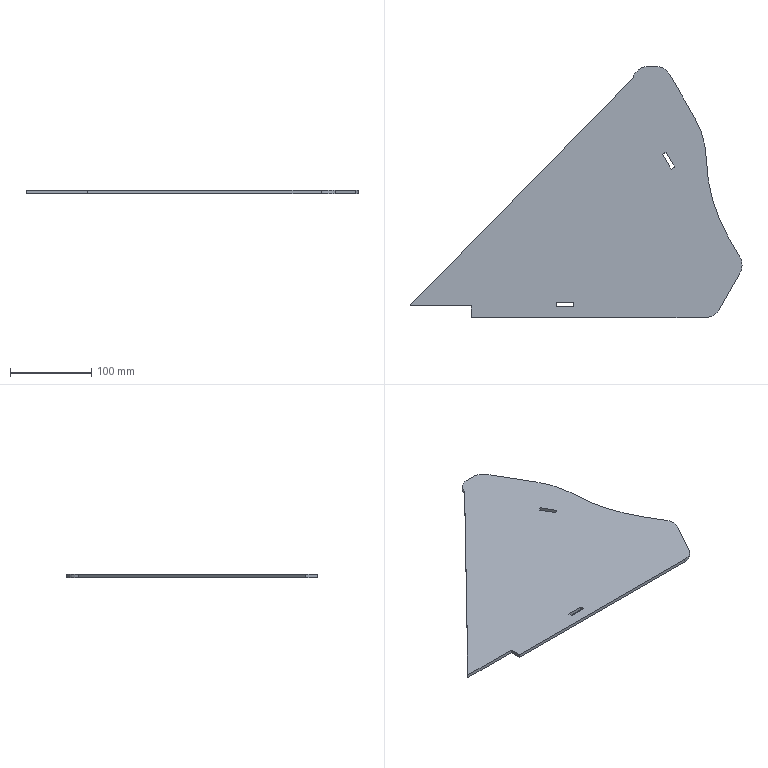Part | SolidWorks | features FlatPattern 1, SMBaseFlange 1, SheetMetal 1 | 1 solid | 25 faces | box 409.722 x 310 x 4 mm | volume 283862 mm3 | plane 18 | cylinder 7 | commonest cylinder face diameters 40 x5 220 x1 400 x1
STEP:
#1=CARTESIAN_POINT('',(421.287,163.625,-4.));
#2=VERTEX_POINT('',#1);
#3=CARTESIAN_POINT('',(423.905,173.519,-4.));
#4=VERTEX_POINT('',#3);
#5=CARTESIAN_POINT('',(403.905,173.519,-4.));
#6=DIRECTION('',(0.,0.,1.));
#7=DIRECTION('',(1.,0.,0.));
#8=AXIS2_PLACEMENT_3D('',#5,#6,#7);
#9=CIRCLE('',#8,20.);
#10=EDGE_CURVE('',#2,#4,#9,.T.);
#11=ORIENTED_EDGE('',*,*,#10,.T.);
#12=CARTESIAN_POINT('',(423.905,173.519,0.));
#13=VERTEX_POINT('',#12);
#14=CARTESIAN_POINT('',(423.905,173.519,-4.));
#15=DIRECTION('',(0.,0.,1.));
#16=VECTOR('',#15,1000.);
#17=LINE('',#14,#16);
#18=EDGE_CURVE('',#4,#13,#17,.T.);
#19=ORIENTED_EDGE('',*,*,#18,.T.);
#20=CARTESIAN_POINT('',(421.287,163.625,0.));
#21=VERTEX_POINT('',#20);
#22=CARTESIAN_POINT('',(403.905,173.519,0.));
#23=DIRECTION('',(0.,0.,1.));
#24=DIRECTION('',(1.,0.,0.));
#25=AXIS2_PLACEMENT_3D('',#22,#23,#24);
#26=CIRCLE('',#25,20.);
#27=EDGE_CURVE('',#21,#13,#26,.T.);
#28=ORIENTED_EDGE('',*,*,#27,.F.);
#29=CARTESIAN_POINT('',(421.287,163.625,-4.));
#30=DIRECTION('',(0.,0.,1.));
#31=VECTOR('',#30,1000.);
#32=LINE('',#29,#31);
#33=EDGE_CURVE('',#2,#21,#32,.T.);
#34=ORIENTED_EDGE('',*,*,#33,.F.);
#35=EDGE_LOOP('',(#11,#19,#28,#34));
#36=FACE_OUTER_BOUND('',#35,.T.);
#37=CARTESIAN_POINT('',(403.905,173.519,-4.));
#38=DIRECTION('',(0.,0.,1.));
#39=DIRECTION('',(1.,0.,0.));
#40=AXIS2_PLACEMENT_3D('',#37,#38,#39);
#41=CYLINDRICAL_SURFACE('',#40,20.);
#42=ADVANCED_FACE('',(#36),#41,.T.);
#43=CARTESIAN_POINT('',(89.973,108.614,0.));
#44=VERTEX_POINT('',#43);
#45=CARTESIAN_POINT('',(378.344,108.614,0.));
#46=VERTEX_POINT('',#45);
#47=CARTESIAN_POINT('',(89.973,108.614,0.));
#48=DIRECTION('',(1.,0.,0.));
#49=VECTOR('',#48,1000.);
#50=LINE('',#47,#49);
#51=EDGE_CURVE('',#44,#46,#50,.T.);
#52=ORIENTED_EDGE('',*,*,#51,.F.);
#53=CARTESIAN_POINT('',(89.973,108.614,-4.));
#54=VERTEX_POINT('',#53);
#55=CARTESIAN_POINT('',(89.973,108.614,-4.));
#56=DIRECTION('',(0.,0.,1.));
#57=VECTOR('',#56,1000.);
#58=LINE('',#55,#57);
#59=EDGE_CURVE('',#54,#44,#58,.T.);
#60=ORIENTED_EDGE('',*,*,#59,.F.);
#61=CARTESIAN_POINT('',(378.344,108.614,-4.));
#62=VERTEX_POINT('',#61);
#63=CARTESIAN_POINT('',(89.973,108.614,-4.));
#64=DIRECTION('',(1.,0.,0.));
#65=VECTOR('',#64,1000.);
#66=LINE('',#63,#65);
#67=EDGE_CURVE('',#54,#62,#66,.T.);
#68=ORIENTED_EDGE('',*,*,#67,.T.);
#69=CARTESIAN_POINT('',(378.344,108.614,-4.));
#70=DIRECTION('',(0.,0.,1.));
#71=VECTOR('',#70,1000.);
#72=LINE('',#69,#71);
#73=EDGE_CURVE('',#62,#46,#72,.T.);
#74=ORIENTED_EDGE('',*,*,#73,.T.);
#75=EDGE_LOOP('',(#52,#60,#68,#74));
#76=FACE_OUTER_BOUND('',#75,.T.);
#77=CARTESIAN_POINT('',(89.973,108.614,-4.));
#78=DIRECTION('',(0.,-1.,0.));
#79=DIRECTION('',(1.,0.,0.));
#80=AXIS2_PLACEMENT_3D('',#77,#78,#79);
#81=PLANE('',#80);
#82=ADVANCED_FACE('',(#76),#81,.T.);
#83=CARTESIAN_POINT('',(89.973,123.114,0.));
#84=VERTEX_POINT('',#83);
#85=CARTESIAN_POINT('',(89.973,108.614,0.));
#86=DIRECTION('',(0.,-1.,0.));
#87=VECTOR('',#86,1000.);
#88=LINE('',#85,#87);
#89=EDGE_CURVE('',#84,#44,#88,.T.);
#90=ORIENTED_EDGE('',*,*,#89,.F.);
#91=CARTESIAN_POINT('',(89.973,123.114,-4.));
#92=VERTEX_POINT('',#91);
#93=CARTESIAN_POINT('',(89.973,123.114,-4.));
#94=DIRECTION('',(0.,0.,1.));
#95=VECTOR('',#94,1000.);
#96=LINE('',#93,#95);
#97=EDGE_CURVE('',#92,#84,#96,.T.);
#98=ORIENTED_EDGE('',*,*,#97,.F.);
#99=CARTESIAN_POINT('',(89.973,108.614,-4.));
#100=DIRECTION('',(0.,-1.,0.));
#101=VECTOR('',#100,1000.);
#102=LINE('',#99,#101);
#103=EDGE_CURVE('',#92,#54,#102,.T.);
#104=ORIENTED_EDGE('',*,*,#103,.T.);
#105=ORIENTED_EDGE('',*,*,#59,.T.);
#106=EDGE_LOOP('',(#90,#98,#104,#105));
#107=FACE_OUTER_BOUND('',#106,.T.);
#108=CARTESIAN_POINT('',(89.973,108.614,-4.));
#109=DIRECTION('',(-1.,0.,0.));
#110=DIRECTION('',(0.,0.,1.));
#111=AXIS2_PLACEMENT_3D('',#108,#109,#110);
#112=PLANE('',#111);
#113=ADVANCED_FACE('',(#107),#112,.T.);
#114=CARTESIAN_POINT('',(14.183,123.114,0.));
#115=VERTEX_POINT('',#114);
#116=CARTESIAN_POINT('',(89.973,123.114,0.));
#117=DIRECTION('',(1.,0.,0.));
#118=VECTOR('',#117,1000.);
#119=LINE('',#116,#118);
#120=EDGE_CURVE('',#115,#84,#119,.T.);
#121=ORIENTED_EDGE('',*,*,#120,.F.);
#122=CARTESIAN_POINT('',(14.183,123.114,-4.));
#123=VERTEX_POINT('',#122);
#124=CARTESIAN_POINT('',(14.183,123.114,-4.));
#125=DIRECTION('',(0.,0.,1.));
#126=VECTOR('',#125,1000.);
#127=LINE('',#124,#126);
#128=EDGE_CURVE('',#123,#115,#127,.T.);
#129=ORIENTED_EDGE('',*,*,#128,.F.);
#130=CARTESIAN_POINT('',(89.973,123.114,-4.));
#131=DIRECTION('',(1.,0.,0.));
#132=VECTOR('',#131,1000.);
#133=LINE('',#130,#132);
#134=EDGE_CURVE('',#123,#92,#133,.T.);
#135=ORIENTED_EDGE('',*,*,#134,.T.);
#136=ORIENTED_EDGE('',*,*,#97,.T.);
#137=EDGE_LOOP('',(#121,#129,#135,#136));
#138=FACE_OUTER_BOUND('',#137,.T.);
#139=CARTESIAN_POINT('',(89.973,123.114,-4.));
#140=DIRECTION('',(0.,-1.,0.));
#141=DIRECTION('',(0.,0.,-1.));
#142=AXIS2_PLACEMENT_3D('',#139,#140,#141);
#143=PLANE('',#142);
#144=ADVANCED_FACE('',(#138),#143,.T.);
#145=CARTESIAN_POINT('',(288.973,403.614,0.));
#146=VERTEX_POINT('',#145);
#147=CARTESIAN_POINT('',(288.973,403.614,0.));
#148=DIRECTION('',(-0.6998,-0.7143,0.));
#149=VECTOR('',#148,1000.);
#150=LINE('',#147,#149);
#151=EDGE_CURVE('',#146,#115,#150,.T.);
#152=ORIENTED_EDGE('',*,*,#151,.F.);
#153=CARTESIAN_POINT('',(288.973,403.614,-4.));
#154=VERTEX_POINT('',#153);
#155=CARTESIAN_POINT('',(288.973,403.614,-4.));
#156=DIRECTION('',(0.,0.,1.));
#157=VECTOR('',#156,1000.);
#158=LINE('',#155,#157);
#159=EDGE_CURVE('',#154,#146,#158,.T.);
#160=ORIENTED_EDGE('',*,*,#159,.F.);
#161=CARTESIAN_POINT('',(288.973,403.614,-4.));
#162=DIRECTION('',(-0.6998,-0.7143,0.));
#163=VECTOR('',#162,1000.);
#164=LINE('',#161,#163);
#165=EDGE_CURVE('',#154,#123,#164,.T.);
#166=ORIENTED_EDGE('',*,*,#165,.T.);
#167=ORIENTED_EDGE('',*,*,#128,.T.);
#168=EDGE_LOOP('',(#152,#160,#166,#167));
#169=FACE_OUTER_BOUND('',#168,.T.);
#170=CARTESIAN_POINT('',(288.973,403.614,-4.));
#171=DIRECTION('',(-0.7143,0.6998,0.));
#172=DIRECTION('',(-0.6998,-0.7143,0.));
#173=AXIS2_PLACEMENT_3D('',#170,#171,#172);
#174=PLANE('',#173);
#175=ADVANCED_FACE('',(#169),#174,.T.);
#176=CARTESIAN_POINT('',(308.338,418.614,0.));
#177=VERTEX_POINT('',#176);
#178=CARTESIAN_POINT('',(308.338,398.614,0.));
#179=DIRECTION('',(0.,0.,1.));
#180=DIRECTION('',(1.,0.,0.));
#181=AXIS2_PLACEMENT_3D('',#178,#179,#180);
#182=CIRCLE('',#181,20.);
#183=EDGE_CURVE('',#177,#146,#182,.T.);
#184=ORIENTED_EDGE('',*,*,#183,.F.);
#185=CARTESIAN_POINT('',(308.338,418.614,-4.));
#186=VERTEX_POINT('',#185);
#187=CARTESIAN_POINT('',(308.338,418.614,-4.));
#188=DIRECTION('',(0.,0.,1.));
#189=VECTOR('',#188,1000.);
#190=LINE('',#187,#189);
#191=EDGE_CURVE('',#186,#177,#190,.T.);
#192=ORIENTED_EDGE('',*,*,#191,.F.);
#193=CARTESIAN_POINT('',(308.338,398.614,-4.));
#194=DIRECTION('',(0.,0.,1.));
#195=DIRECTION('',(1.,0.,0.));
#196=AXIS2_PLACEMENT_3D('',#193,#194,#195);
#197=CIRCLE('',#196,20.);
#198=EDGE_CURVE('',#186,#154,#197,.T.);
#199=ORIENTED_EDGE('',*,*,#198,.T.);
#200=ORIENTED_EDGE('',*,*,#159,.T.);
#201=EDGE_LOOP('',(#184,#192,#199,#200));
#202=FACE_OUTER_BOUND('',#201,.T.);
#203=CARTESIAN_POINT('',(308.338,398.614,-4.));
#204=DIRECTION('',(0.,0.,1.));
#205=DIRECTION('',(1.,0.,0.));
#206=AXIS2_PLACEMENT_3D('',#203,#204,#205);
#207=CYLINDRICAL_SURFACE('',#206,20.);
#208=ADVANCED_FACE('',(#202),#207,.T.);
#209=CARTESIAN_POINT('',(317.426,418.614,0.));
#210=VERTEX_POINT('',#209);
#211=CARTESIAN_POINT('',(317.426,418.614,0.));
#212=DIRECTION('',(-1.,0.,0.));
#213=VECTOR('',#212,1000.);
#214=LINE('',#211,#213);
#215=EDGE_CURVE('',#210,#177,#214,.T.);
#216=ORIENTED_EDGE('',*,*,#215,.F.);
#217=CARTESIAN_POINT('',(317.426,418.614,-4.));
#218=VERTEX_POINT('',#217);
#219=CARTESIAN_POINT('',(317.426,418.614,-4.));
#220=DIRECTION('',(0.,0.,1.));
#221=VECTOR('',#220,1000.);
#222=LINE('',#219,#221);
#223=EDGE_CURVE('',#218,#210,#222,.T.);
#224=ORIENTED_EDGE('',*,*,#223,.F.);
#225=CARTESIAN_POINT('',(317.426,418.614,-4.));
#226=DIRECTION('',(-1.,0.,0.));
#227=VECTOR('',#226,1000.);
#228=LINE('',#225,#227);
#229=EDGE_CURVE('',#218,#186,#228,.T.);
#230=ORIENTED_EDGE('',*,*,#229,.T.);
#231=ORIENTED_EDGE('',*,*,#191,.T.);
#232=EDGE_LOOP('',(#216,#224,#230,#231));
#233=FACE_OUTER_BOUND('',#232,.T.);
#234=CARTESIAN_POINT('',(317.426,418.614,-4.));
#235=DIRECTION('',(0.,1.,0.));
#236=DIRECTION('',(0.,0.,1.));
#237=AXIS2_PLACEMENT_3D('',#234,#235,#236);
#238=PLANE('',#237);
#239=ADVANCED_FACE('',(#233),#238,.T.);
#240=CARTESIAN_POINT('',(334.746,408.614,0.));
#241=VERTEX_POINT('',#240);
#242=CARTESIAN_POINT('',(317.426,398.614,0.));
#243=DIRECTION('',(0.,0.,1.));
#244=DIRECTION('',(1.,0.,0.));
#245=AXIS2_PLACEMENT_3D('',#242,#243,#244);
#246=CIRCLE('',#245,20.);
#247=EDGE_CURVE('',#241,#210,#246,.T.);
#248=ORIENTED_EDGE('',*,*,#247,.F.);
#249=CARTESIAN_POINT('',(334.746,408.614,-4.));
#250=VERTEX_POINT('',#249);
#251=CARTESIAN_POINT('',(334.746,408.614,-4.));
#252=DIRECTION('',(0.,0.,1.));
#253=VECTOR('',#252,1000.);
#254=LINE('',#251,#253);
#255=EDGE_CURVE('',#250,#241,#254,.T.);
#256=ORIENTED_EDGE('',*,*,#255,.F.);
#257=CARTESIAN_POINT('',(317.426,398.614,-4.));
#258=DIRECTION('',(0.,0.,1.));
#259=DIRECTION('',(1.,0.,0.));
#260=AXIS2_PLACEMENT_3D('',#257,#258,#259);
#261=CIRCLE('',#260,20.);
#262=EDGE_CURVE('',#250,#218,#261,.T.);
#263=ORIENTED_EDGE('',*,*,#262,.T.);
#264=ORIENTED_EDGE('',*,*,#223,.T.);
#265=EDGE_LOOP('',(#248,#256,#263,#264));
#266=FACE_OUTER_BOUND('',#265,.T.);
#267=CARTESIAN_POINT('',(317.426,398.614,-4.));
#268=DIRECTION('',(0.,0.,1.));
#269=DIRECTION('',(1.,0.,0.));
#270=AXIS2_PLACEMENT_3D('',#267,#268,#269);
#271=CYLINDRICAL_SURFACE('',#270,20.);
#272=ADVANCED_FACE('',(#266),#271,.T.);
#273=CARTESIAN_POINT('',(365.332,355.639,0.));
#274=VERTEX_POINT('',#273);
#275=CARTESIAN_POINT('',(365.332,355.639,0.));
#276=DIRECTION('',(-0.5,0.866,0.));
#277=VECTOR('',#276,1000.);
#278=LINE('',#275,#277);
#279=EDGE_CURVE('',#274,#241,#278,.T.);
#280=ORIENTED_EDGE('',*,*,#279,.F.);
#281=CARTESIAN_POINT('',(365.332,355.639,-4.));
#282=VERTEX_POINT('',#281);
#283=CARTESIAN_POINT('',(365.332,355.639,-4.));
#284=DIRECTION('',(0.,0.,1.));
#285=VECTOR('',#284,1000.);
#286=LINE('',#283,#285);
#287=EDGE_CURVE('',#282,#274,#286,.T.);
#288=ORIENTED_EDGE('',*,*,#287,.F.);
#289=CARTESIAN_POINT('',(365.332,355.639,-4.));
#290=DIRECTION('',(-0.5,0.866,0.));
#291=VECTOR('',#290,1000.);
#292=LINE('',#289,#291);
#293=EDGE_CURVE('',#282,#250,#292,.T.);
#294=ORIENTED_EDGE('',*,*,#293,.T.);
#295=ORIENTED_EDGE('',*,*,#255,.T.);
#296=EDGE_LOOP('',(#280,#288,#294,#295));
#297=FACE_OUTER_BOUND('',#296,.T.);
#298=CARTESIAN_POINT('',(365.332,355.639,-4.));
#299=DIRECTION('',(0.866,0.5,0.));
#300=DIRECTION('',(-0.5,0.866,0.));
#301=AXIS2_PLACEMENT_3D('',#298,#299,#300);
#302=PLANE('',#301);
#303=ADVANCED_FACE('',(#297),#302,.T.);
#304=CARTESIAN_POINT('',(380.035,303.4,0.));
#305=VERTEX_POINT('',#304);
#306=CARTESIAN_POINT('',(270.069,300.639,0.));
#307=DIRECTION('',(0.,0.,1.));
#308=DIRECTION('',(1.,0.,0.));
#309=AXIS2_PLACEMENT_3D('',#306,#307,#308);
#310=CIRCLE('',#309,110.);
#311=EDGE_CURVE('',#305,#274,#310,.T.);
#312=ORIENTED_EDGE('',*,*,#311,.F.);
#313=CARTESIAN_POINT('',(380.035,303.4,-4.));
#314=VERTEX_POINT('',#313);
#315=CARTESIAN_POINT('',(380.035,303.4,-4.));
#316=DIRECTION('',(0.,0.,1.));
#317=VECTOR('',#316,1000.);
#318=LINE('',#315,#317);
#319=EDGE_CURVE('',#314,#305,#318,.T.);
#320=ORIENTED_EDGE('',*,*,#319,.F.);
#321=CARTESIAN_POINT('',(270.069,300.639,-4.));
#322=DIRECTION('',(0.,0.,1.));
#323=DIRECTION('',(1.,0.,0.));
#324=AXIS2_PLACEMENT_3D('',#321,#322,#323);
#325=CIRCLE('',#324,110.);
#326=EDGE_CURVE('',#314,#282,#325,.T.);
#327=ORIENTED_EDGE('',*,*,#326,.T.);
#328=ORIENTED_EDGE('',*,*,#287,.T.);
#329=EDGE_LOOP('',(#312,#320,#327,#328));
#330=FACE_OUTER_BOUND('',#329,.T.);
#331=CARTESIAN_POINT('',(270.069,300.639,-4.));
#332=DIRECTION('',(0.,0.,1.));
#333=DIRECTION('',(1.,0.,0.));
#334=AXIS2_PLACEMENT_3D('',#331,#332,#333);
#335=CYLINDRICAL_SURFACE('',#334,110.);
#336=ADVANCED_FACE('',(#330),#335,.T.);
#337=CARTESIAN_POINT('',(406.983,208.065,0.));
#338=VERTEX_POINT('',#337);
#339=CARTESIAN_POINT('',(579.971,308.44,0.));
#340=DIRECTION('',(0.,0.,-1.));
#341=DIRECTION('',(1.,0.,0.));
#342=AXIS2_PLACEMENT_3D('',#339,#340,#341);
#343=CIRCLE('',#342,200.);
#344=EDGE_CURVE('',#338,#305,#343,.T.);
#345=ORIENTED_EDGE('',*,*,#344,.F.);
#346=CARTESIAN_POINT('',(406.983,208.065,-4.));
#347=VERTEX_POINT('',#346);
#348=CARTESIAN_POINT('',(406.983,208.065,-4.));
#349=DIRECTION('',(0.,0.,1.));
#350=VECTOR('',#349,1000.);
#351=LINE('',#348,#350);
#352=EDGE_CURVE('',#347,#338,#351,.T.);
#353=ORIENTED_EDGE('',*,*,#352,.F.);
#354=CARTESIAN_POINT('',(579.971,308.44,-4.));
#355=DIRECTION('',(0.,0.,-1.));
#356=DIRECTION('',(1.,0.,0.));
#357=AXIS2_PLACEMENT_3D('',#354,#355,#356);
#358=CIRCLE('',#357,200.);
#359=EDGE_CURVE('',#347,#314,#358,.T.);
#360=ORIENTED_EDGE('',*,*,#359,.T.);
#361=ORIENTED_EDGE('',*,*,#319,.T.);
#362=EDGE_LOOP('',(#345,#353,#360,#361));
#363=FACE_OUTER_BOUND('',#362,.T.);
#364=CARTESIAN_POINT('',(579.971,308.44,-4.));
#365=DIRECTION('',(0.,0.,1.));
#366=DIRECTION('',(1.,0.,0.));
#367=AXIS2_PLACEMENT_3D('',#364,#365,#366);
#368=CYLINDRICAL_SURFACE('',#367,200.);
#369=ADVANCED_FACE('',(#363),#368,.F.);
#370=CARTESIAN_POINT('',(421.204,183.556,0.));
#371=VERTEX_POINT('',#370);
#372=CARTESIAN_POINT('',(421.204,183.556,0.));
#373=DIRECTION('',(-0.5019,0.8649,0.));
#374=VECTOR('',#373,1000.);
#375=LINE('',#372,#374);
#376=EDGE_CURVE('',#371,#338,#375,.T.);
#377=ORIENTED_EDGE('',*,*,#376,.F.);
#378=CARTESIAN_POINT('',(421.204,183.556,-4.));
#379=VERTEX_POINT('',#378);
#380=CARTESIAN_POINT('',(421.204,183.556,-4.));
#381=DIRECTION('',(0.,0.,1.));
#382=VECTOR('',#381,1000.);
#383=LINE('',#380,#382);
#384=EDGE_CURVE('',#379,#371,#383,.T.);
#385=ORIENTED_EDGE('',*,*,#384,.F.);
#386=CARTESIAN_POINT('',(421.204,183.556,-4.));
#387=DIRECTION('',(-0.5019,0.8649,0.));
#388=VECTOR('',#387,1000.);
#389=LINE('',#386,#388);
#390=EDGE_CURVE('',#379,#347,#389,.T.);
#391=ORIENTED_EDGE('',*,*,#390,.T.);
#392=ORIENTED_EDGE('',*,*,#352,.T.);
#393=EDGE_LOOP('',(#377,#385,#391,#392));
#394=FACE_OUTER_BOUND('',#393,.T.);
#395=CARTESIAN_POINT('',(421.204,183.556,-4.));
#396=DIRECTION('',(0.8649,0.5019,0.));
#397=DIRECTION('',(-0.5019,0.8649,0.));
#398=AXIS2_PLACEMENT_3D('',#395,#396,#397);
#399=PLANE('',#398);
#400=ADVANCED_FACE('',(#394),#399,.T.);
#401=ORIENTED_EDGE('',*,*,#18,.F.);
#402=CARTESIAN_POINT('',(403.905,173.519,-4.));
#403=DIRECTION('',(0.,0.,1.));
#404=DIRECTION('',(1.,0.,0.));
#405=AXIS2_PLACEMENT_3D('',#402,#403,#404);
#406=CIRCLE('',#405,20.);
#407=EDGE_CURVE('',#4,#379,#406,.T.);
#408=ORIENTED_EDGE('',*,*,#407,.T.);
#409=ORIENTED_EDGE('',*,*,#384,.T.);
#410=CARTESIAN_POINT('',(403.905,173.519,0.));
#411=DIRECTION('',(0.,0.,1.));
#412=DIRECTION('',(1.,0.,0.));
#413=AXIS2_PLACEMENT_3D('',#410,#411,#412);
#414=CIRCLE('',#413,20.);
#415=EDGE_CURVE('',#13,#371,#414,.T.);
#416=ORIENTED_EDGE('',*,*,#415,.F.);
#417=EDGE_LOOP('',(#401,#408,#409,#416));
#418=FACE_OUTER_BOUND('',#417,.T.);
#419=CARTESIAN_POINT('',(403.905,173.519,-4.));
#420=DIRECTION('',(0.,0.,1.));
#421=DIRECTION('',(1.,0.,0.));
#422=AXIS2_PLACEMENT_3D('',#419,#420,#421);
#423=CYLINDRICAL_SURFACE('',#422,20.);
#424=ADVANCED_FACE('',(#418),#423,.T.);
#425=CARTESIAN_POINT('',(395.726,118.72,0.));
#426=VERTEX_POINT('',#425);
#427=CARTESIAN_POINT('',(395.726,118.72,0.));
#428=DIRECTION('',(0.4947,0.8691,0.));
#429=VECTOR('',#428,1000.);
#430=LINE('',#427,#429);
#431=EDGE_CURVE('',#426,#21,#430,.T.);
#432=ORIENTED_EDGE('',*,*,#431,.F.);
#433=CARTESIAN_POINT('',(395.726,118.72,-4.));
#434=VERTEX_POINT('',#433);
#435=CARTESIAN_POINT('',(395.726,118.72,-4.));
#436=DIRECTION('',(0.,0.,1.));
#437=VECTOR('',#436,1000.);
#438=LINE('',#435,#437);
#439=EDGE_CURVE('',#434,#426,#438,.T.);
#440=ORIENTED_EDGE('',*,*,#439,.F.);
#441=CARTESIAN_POINT('',(395.726,118.72,-4.));
#442=DIRECTION('',(0.4947,0.8691,0.));
#443=VECTOR('',#442,1000.);
#444=LINE('',#441,#443);
#445=EDGE_CURVE('',#434,#2,#444,.T.);
#446=ORIENTED_EDGE('',*,*,#445,.T.);
#447=ORIENTED_EDGE('',*,*,#33,.T.);
#448=EDGE_LOOP('',(#432,#440,#446,#447));
#449=FACE_OUTER_BOUND('',#448,.T.);
#450=CARTESIAN_POINT('',(395.726,118.72,-4.));
#451=DIRECTION('',(0.8691,-0.4947,0.));
#452=DIRECTION('',(0.4947,0.8691,0.));
#453=AXIS2_PLACEMENT_3D('',#450,#451,#452);
#454=PLANE('',#453);
#455=ADVANCED_FACE('',(#449),#454,.T.);
#456=CARTESIAN_POINT('',(378.344,128.614,0.));
#457=DIRECTION('',(0.,0.,1.));
#458=DIRECTION('',(1.,0.,0.));
#459=AXIS2_PLACEMENT_3D('',#456,#457,#458);
#460=CIRCLE('',#459,20.);
#461=EDGE_CURVE('',#46,#426,#460,.T.);
#462=ORIENTED_EDGE('',*,*,#461,.F.);
#463=ORIENTED_EDGE('',*,*,#73,.F.);
#464=CARTESIAN_POINT('',(378.344,128.614,-4.));
#465=DIRECTION('',(0.,0.,1.));
#466=DIRECTION('',(1.,0.,0.));
#467=AXIS2_PLACEMENT_3D('',#464,#465,#466);
#468=CIRCLE('',#467,20.);
#469=EDGE_CURVE('',#62,#434,#468,.T.);
#470=ORIENTED_EDGE('',*,*,#469,.T.);
#471=ORIENTED_EDGE('',*,*,#439,.T.);
#472=EDGE_LOOP('',(#462,#463,#470,#471));
#473=FACE_OUTER_BOUND('',#472,.T.);
#474=CARTESIAN_POINT('',(378.344,128.614,-4.));
#475=DIRECTION('',(0.,0.,1.));
#476=DIRECTION('',(1.,0.,0.));
#477=AXIS2_PLACEMENT_3D('',#474,#475,#476);
#478=CYLINDRICAL_SURFACE('',#477,20.);
#479=ADVANCED_FACE('',(#473),#478,.T.);
#480=CARTESIAN_POINT('',(215.478,127.114,-4.));
#481=VERTEX_POINT('',#480);
#482=CARTESIAN_POINT('',(194.478,127.114,-4.));
#483=VERTEX_POINT('',#482);
#484=CARTESIAN_POINT('',(215.478,127.114,-4.));
#485=DIRECTION('',(-1.,0.,0.));
#486=VECTOR('',#485,1000.);
#487=LINE('',#484,#486);
#488=EDGE_CURVE('',#481,#483,#487,.T.);
#489=ORIENTED_EDGE('',*,*,#488,.T.);
#490=CARTESIAN_POINT('',(194.478,122.114,-4.));
#491=VERTEX_POINT('',#490);
#492=CARTESIAN_POINT('',(194.478,127.114,-4.));
#493=DIRECTION('',(0.,-1.,0.));
#494=VECTOR('',#493,1000.);
#495=LINE('',#492,#494);
#496=EDGE_CURVE('',#483,#491,#495,.T.);
#497=ORIENTED_EDGE('',*,*,#496,.T.);
#498=CARTESIAN_POINT('',(215.478,122.114,-4.));
#499=VERTEX_POINT('',#498);
#500=CARTESIAN_POINT('',(194.478,122.114,-4.));
#501=DIRECTION('',(1.,0.,0.));
#502=VECTOR('',#501,1000.);
#503=LINE('',#500,#502);
#504=EDGE_CURVE('',#491,#499,#503,.T.);
#505=ORIENTED_EDGE('',*,*,#504,.T.);
#506=CARTESIAN_POINT('',(215.478,122.114,-4.));
#507=DIRECTION('',(0.,1.,0.));
#508=VECTOR('',#507,1000.);
#509=LINE('',#506,#508);
#510=EDGE_CURVE('',#499,#481,#509,.T.);
#511=ORIENTED_EDGE('',*,*,#510,.T.);
#512=EDGE_LOOP('',(#489,#497,#505,#511));
#513=FACE_BOUND('',#512,.T.);
#514=CARTESIAN_POINT('',(330.283,312.574,-4.));
#515=VERTEX_POINT('',#514);
#516=CARTESIAN_POINT('',(325.953,310.074,-4.));
#517=VERTEX_POINT('',#516);
#518=CARTESIAN_POINT('',(330.283,312.574,-4.));
#519=DIRECTION('',(-0.866,-0.5,0.));
#520=VECTOR('',#519,1000.);
#521=LINE('',#518,#520);
#522=EDGE_CURVE('',#515,#517,#521,.T.);
#523=ORIENTED_EDGE('',*,*,#522,.T.);
#524=CARTESIAN_POINT('',(336.453,291.888,-4.));
#525=VERTEX_POINT('',#524);
#526=CARTESIAN_POINT('',(325.953,310.074,-4.));
#527=DIRECTION('',(0.5,-0.866,0.));
#528=VECTOR('',#527,1000.);
#529=LINE('',#526,#528);
#530=EDGE_CURVE('',#517,#525,#529,.T.);
#531=ORIENTED_EDGE('',*,*,#530,.T.);
#532=CARTESIAN_POINT('',(340.783,294.388,-4.));
#533=VERTEX_POINT('',#532);
#534=CARTESIAN_POINT('',(336.453,291.888,-4.));
#535=DIRECTION('',(0.866,0.5,0.));
#536=VECTOR('',#535,1000.);
#537=LINE('',#534,#536);
#538=EDGE_CURVE('',#525,#533,#537,.T.);
#539=ORIENTED_EDGE('',*,*,#538,.T.);
#540=CARTESIAN_POINT('',(340.783,294.388,-4.));
#541=DIRECTION('',(-0.5,0.866,0.));
#542=VECTOR('',#541,1000.);
#543=LINE('',#540,#542);
#544=EDGE_CURVE('',#533,#515,#543,.T.);
#545=ORIENTED_EDGE('',*,*,#544,.T.);
#546=EDGE_LOOP('',(#523,#531,#539,#545));
#547=FACE_BOUND('',#546,.T.);
#548=ORIENTED_EDGE('',*,*,#67,.F.);
#549=ORIENTED_EDGE('',*,*,#103,.F.);
#550=ORIENTED_EDGE('',*,*,#134,.F.);
#551=ORIENTED_EDGE('',*,*,#165,.F.);
#552=ORIENTED_EDGE('',*,*,#198,.F.);
#553=ORIENTED_EDGE('',*,*,#229,.F.);
#554=ORIENTED_EDGE('',*,*,#262,.F.);
#555=ORIENTED_EDGE('',*,*,#293,.F.);
#556=ORIENTED_EDGE('',*,*,#326,.F.);
#557=ORIENTED_EDGE('',*,*,#359,.F.);
#558=ORIENTED_EDGE('',*,*,#390,.F.);
#559=ORIENTED_EDGE('',*,*,#407,.F.);
#560=ORIENTED_EDGE('',*,*,#10,.F.);
#561=ORIENTED_EDGE('',*,*,#445,.F.);
#562=ORIENTED_EDGE('',*,*,#469,.F.);
#563=EDGE_LOOP('',(#548,#549,#550,#551,#552,#553,#554,#555,#556,#557,#558,#559,#560,#561,#562));
#564=FACE_OUTER_BOUND('',#563,.T.);
#565=CARTESIAN_POINT('',(378.344,128.614,-4.));
#566=DIRECTION('',(0.,0.,1.));
#567=DIRECTION('',(1.,0.,0.));
#568=AXIS2_PLACEMENT_3D('',#565,#566,#567);
#569=PLANE('',#568);
#570=ADVANCED_FACE('',(#513,#547,#564),#569,.F.);
#571=CARTESIAN_POINT('',(194.478,127.114,0.));
#572=VERTEX_POINT('',#571);
#573=CARTESIAN_POINT('',(194.478,122.114,0.));
#574=VERTEX_POINT('',#573);
#575=CARTESIAN_POINT('',(194.478,127.114,0.));
#576=DIRECTION('',(0.,-1.,0.));
#577=VECTOR('',#576,1000.);
#578=LINE('',#575,#577);
#579=EDGE_CURVE('',#572,#574,#578,.T.);
#580=ORIENTED_EDGE('',*,*,#579,.F.);
#581=CARTESIAN_POINT('',(215.478,127.114,0.));
#582=VERTEX_POINT('',#581);
#583=CARTESIAN_POINT('',(215.478,127.114,0.));
#584=DIRECTION('',(-1.,0.,0.));
#585=VECTOR('',#584,1000.);
#586=LINE('',#583,#585);
#587=EDGE_CURVE('',#582,#572,#586,.T.);
#588=ORIENTED_EDGE('',*,*,#587,.F.);
#589=CARTESIAN_POINT('',(215.478,122.114,0.));
#590=VERTEX_POINT('',#589);
#591=CARTESIAN_POINT('',(215.478,122.114,0.));
#592=DIRECTION('',(0.,1.,0.));
#593=VECTOR('',#592,1000.);
#594=LINE('',#591,#593);
#595=EDGE_CURVE('',#590,#582,#594,.T.);
#596=ORIENTED_EDGE('',*,*,#595,.F.);
#597=CARTESIAN_POINT('',(194.478,122.114,0.));
#598=DIRECTION('',(1.,0.,0.));
#599=VECTOR('',#598,1000.);
#600=LINE('',#597,#599);
#601=EDGE_CURVE('',#574,#590,#600,.T.);
#602=ORIENTED_EDGE('',*,*,#601,.F.);
#603=EDGE_LOOP('',(#580,#588,#596,#602));
#604=FACE_BOUND('',#603,.T.);
#605=CARTESIAN_POINT('',(325.953,310.074,0.));
#606=VERTEX_POINT('',#605);
#607=CARTESIAN_POINT('',(336.453,291.888,0.));
#608=VERTEX_POINT('',#607);
#609=CARTESIAN_POINT('',(325.953,310.074,0.));
#610=DIRECTION('',(0.5,-0.866,0.));
#611=VECTOR('',#610,1000.);
#612=LINE('',#609,#611);
#613=EDGE_CURVE('',#606,#608,#612,.T.);
#614=ORIENTED_EDGE('',*,*,#613,.F.);
#615=CARTESIAN_POINT('',(330.283,312.574,0.));
#616=VERTEX_POINT('',#615);
#617=CARTESIAN_POINT('',(330.283,312.574,0.));
#618=DIRECTION('',(-0.866,-0.5,0.));
#619=VECTOR('',#618,1000.);
#620=LINE('',#617,#619);
#621=EDGE_CURVE('',#616,#606,#620,.T.);
#622=ORIENTED_EDGE('',*,*,#621,.F.);
#623=CARTESIAN_POINT('',(340.783,294.388,0.));
#624=VERTEX_POINT('',#623);
#625=CARTESIAN_POINT('',(340.783,294.388,0.));
#626=DIRECTION('',(-0.5,0.866,0.));
#627=VECTOR('',#626,1000.);
#628=LINE('',#625,#627);
#629=EDGE_CURVE('',#624,#616,#628,.T.);
#630=ORIENTED_EDGE('',*,*,#629,.F.);
#631=CARTESIAN_POINT('',(336.453,291.888,0.));
#632=DIRECTION('',(0.866,0.5,0.));
#633=VECTOR('',#632,1000.);
#634=LINE('',#631,#633);
#635=EDGE_CURVE('',#608,#624,#634,.T.);
#636=ORIENTED_EDGE('',*,*,#635,.F.);
#637=EDGE_LOOP('',(#614,#622,#630,#636));
#638=FACE_BOUND('',#637,.T.);
#639=ORIENTED_EDGE('',*,*,#51,.T.);
#640=ORIENTED_EDGE('',*,*,#461,.T.);
#641=ORIENTED_EDGE('',*,*,#431,.T.);
#642=ORIENTED_EDGE('',*,*,#27,.T.);
#643=ORIENTED_EDGE('',*,*,#415,.T.);
#644=ORIENTED_EDGE('',*,*,#376,.T.);
#645=ORIENTED_EDGE('',*,*,#344,.T.);
#646=ORIENTED_EDGE('',*,*,#311,.T.);
#647=ORIENTED_EDGE('',*,*,#279,.T.);
#648=ORIENTED_EDGE('',*,*,#247,.T.);
#649=ORIENTED_EDGE('',*,*,#215,.T.);
#650=ORIENTED_EDGE('',*,*,#183,.T.);
#651=ORIENTED_EDGE('',*,*,#151,.T.);
#652=ORIENTED_EDGE('',*,*,#120,.T.);
#653=ORIENTED_EDGE('',*,*,#89,.T.);
#654=EDGE_LOOP('',(#639,#640,#641,#642,#643,#644,#645,#646,#647,#648,#649,#650,#651,#652,#653));
#655=FACE_OUTER_BOUND('',#654,.T.);
#656=CARTESIAN_POINT('',(378.344,128.614,0.));
#657=DIRECTION('',(0.,0.,1.));
#658=DIRECTION('',(1.,0.,0.));
#659=AXIS2_PLACEMENT_3D('',#656,#657,#658);
#660=PLANE('',#659);
#661=ADVANCED_FACE('',(#604,#638,#655),#660,.T.);
#662=ORIENTED_EDGE('',*,*,#613,.T.);
#663=CARTESIAN_POINT('',(336.453,291.888,-4.));
#664=DIRECTION('',(0.,0.,1.));
#665=VECTOR('',#664,1000.);
#666=LINE('',#663,#665);
#667=EDGE_CURVE('',#525,#608,#666,.T.);
#668=ORIENTED_EDGE('',*,*,#667,.F.);
#669=ORIENTED_EDGE('',*,*,#530,.F.);
#670=CARTESIAN_POINT('',(325.953,310.074,-4.));
#671=DIRECTION('',(0.,0.,1.));
#672=VECTOR('',#671,1000.);
#673=LINE('',#670,#672);
#674=EDGE_CURVE('',#517,#606,#673,.T.);
#675=ORIENTED_EDGE('',*,*,#674,.T.);
#676=EDGE_LOOP('',(#662,#668,#669,#675));
#677=FACE_OUTER_BOUND('',#676,.T.);
#678=CARTESIAN_POINT('',(325.953,310.074,-4.));
#679=DIRECTION('',(-0.866,-0.5,0.));
#680=DIRECTION('',(0.5,-0.866,0.));
#681=AXIS2_PLACEMENT_3D('',#678,#679,#680);
#682=PLANE('',#681);
#683=ADVANCED_FACE('',(#677),#682,.F.);
#684=ORIENTED_EDGE('',*,*,#621,.T.);
#685=ORIENTED_EDGE('',*,*,#674,.F.);
#686=ORIENTED_EDGE('',*,*,#522,.F.);
#687=CARTESIAN_POINT('',(330.283,312.574,-4.));
#688=DIRECTION('',(0.,0.,1.));
#689=VECTOR('',#688,1000.);
#690=LINE('',#687,#689);
#691=EDGE_CURVE('',#515,#616,#690,.T.);
#692=ORIENTED_EDGE('',*,*,#691,.T.);
#693=EDGE_LOOP('',(#684,#685,#686,#692));
#694=FACE_OUTER_BOUND('',#693,.T.);
#695=CARTESIAN_POINT('',(330.283,312.574,-4.));
#696=DIRECTION('',(-0.5,0.866,0.));
#697=DIRECTION('',(-0.866,-0.5,0.));
#698=AXIS2_PLACEMENT_3D('',#695,#696,#697);
#699=PLANE('',#698);
#700=ADVANCED_FACE('',(#694),#699,.F.);
#701=ORIENTED_EDGE('',*,*,#629,.T.);
#702=ORIENTED_EDGE('',*,*,#691,.F.);
#703=ORIENTED_EDGE('',*,*,#544,.F.);
#704=CARTESIAN_POINT('',(340.783,294.388,-4.));
#705=DIRECTION('',(0.,0.,1.));
#706=VECTOR('',#705,1000.);
#707=LINE('',#704,#706);
#708=EDGE_CURVE('',#533,#624,#707,.T.);
#709=ORIENTED_EDGE('',*,*,#708,.T.);
#710=EDGE_LOOP('',(#701,#702,#703,#709));
#711=FACE_OUTER_BOUND('',#710,.T.);
#712=CARTESIAN_POINT('',(340.783,294.388,-4.));
#713=DIRECTION('',(0.866,0.5,0.));
#714=DIRECTION('',(-0.5,0.866,0.));
#715=AXIS2_PLACEMENT_3D('',#712,#713,#714);
#716=PLANE('',#715);
#717=ADVANCED_FACE('',(#711),#716,.F.);
#718=ORIENTED_EDGE('',*,*,#635,.T.);
#719=ORIENTED_EDGE('',*,*,#708,.F.);
#720=ORIENTED_EDGE('',*,*,#538,.F.);
#721=ORIENTED_EDGE('',*,*,#667,.T.);
#722=EDGE_LOOP('',(#718,#719,#720,#721));
#723=FACE_OUTER_BOUND('',#722,.T.);
#724=CARTESIAN_POINT('',(336.453,291.888,-4.));
#725=DIRECTION('',(0.5,-0.866,0.));
#726=DIRECTION('',(0.866,0.5,0.));
#727=AXIS2_PLACEMENT_3D('',#724,#725,#726);
#728=PLANE('',#727);
#729=ADVANCED_FACE('',(#723),#728,.F.);
#730=ORIENTED_EDGE('',*,*,#579,.T.);
#731=CARTESIAN_POINT('',(194.478,122.114,-4.));
#732=DIRECTION('',(0.,0.,1.));
#733=VECTOR('',#732,1000.);
#734=LINE('',#731,#733);
#735=EDGE_CURVE('',#491,#574,#734,.T.);
#736=ORIENTED_EDGE('',*,*,#735,.F.);
#737=ORIENTED_EDGE('',*,*,#496,.F.);
#738=CARTESIAN_POINT('',(194.478,127.114,-4.));
#739=DIRECTION('',(0.,0.,1.));
#740=VECTOR('',#739,1000.);
#741=LINE('',#738,#740);
#742=EDGE_CURVE('',#483,#572,#741,.T.);
#743=ORIENTED_EDGE('',*,*,#742,.T.);
#744=EDGE_LOOP('',(#730,#736,#737,#743));
#745=FACE_OUTER_BOUND('',#744,.T.);
#746=CARTESIAN_POINT('',(194.478,127.114,-4.));
#747=DIRECTION('',(-1.,0.,0.));
#748=DIRECTION('',(0.,0.,1.));
#749=AXIS2_PLACEMENT_3D('',#746,#747,#748);
#750=PLANE('',#749);
#751=ADVANCED_FACE('',(#745),#750,.F.);
#752=ORIENTED_EDGE('',*,*,#587,.T.);
#753=ORIENTED_EDGE('',*,*,#742,.F.);
#754=ORIENTED_EDGE('',*,*,#488,.F.);
#755=CARTESIAN_POINT('',(215.478,127.114,-4.));
#756=DIRECTION('',(0.,0.,1.));
#757=VECTOR('',#756,1000.);
#758=LINE('',#755,#757);
#759=EDGE_CURVE('',#481,#582,#758,.T.);
#760=ORIENTED_EDGE('',*,*,#759,.T.);
#761=EDGE_LOOP('',(#752,#753,#754,#760));
#762=FACE_OUTER_BOUND('',#761,.T.);
#763=CARTESIAN_POINT('',(215.478,127.114,-4.));
#764=DIRECTION('',(0.,1.,0.));
#765=DIRECTION('',(0.,0.,1.));
#766=AXIS2_PLACEMENT_3D('',#763,#764,#765);
#767=PLANE('',#766);
#768=ADVANCED_FACE('',(#762),#767,.F.);
#769=ORIENTED_EDGE('',*,*,#595,.T.);
#770=ORIENTED_EDGE('',*,*,#759,.F.);
#771=ORIENTED_EDGE('',*,*,#510,.F.);
#772=CARTESIAN_POINT('',(215.478,122.114,-4.));
#773=DIRECTION('',(0.,0.,1.));
#774=VECTOR('',#773,1000.);
#775=LINE('',#772,#774);
#776=EDGE_CURVE('',#499,#590,#775,.T.);
#777=ORIENTED_EDGE('',*,*,#776,.T.);
#778=EDGE_LOOP('',(#769,#770,#771,#777));
#779=FACE_OUTER_BOUND('',#778,.T.);
#780=CARTESIAN_POINT('',(215.478,122.114,-4.));
#781=DIRECTION('',(1.,0.,0.));
#782=DIRECTION('',(0.,0.,-1.));
#783=AXIS2_PLACEMENT_3D('',#780,#781,#782);
#784=PLANE('',#783);
#785=ADVANCED_FACE('',(#779),#784,.F.);
#786=ORIENTED_EDGE('',*,*,#601,.T.);
#787=ORIENTED_EDGE('',*,*,#776,.F.);
#788=ORIENTED_EDGE('',*,*,#504,.F.);
#789=ORIENTED_EDGE('',*,*,#735,.T.);
#790=EDGE_LOOP('',(#786,#787,#788,#789));
#791=FACE_OUTER_BOUND('',#790,.T.);
#792=CARTESIAN_POINT('',(194.478,122.114,-4.));
#793=DIRECTION('',(0.,-1.,0.));
#794=DIRECTION('',(0.,0.,-1.));
#795=AXIS2_PLACEMENT_3D('',#792,#793,#794);
#796=PLANE('',#795);
#797=ADVANCED_FACE('',(#791),#796,.F.);
#798=CLOSED_SHELL('',(#42,#82,#113,#144,#175,#208,#239,#272,#303,#336,#369,#400,#424,#455,#479,#570,#661,#683,#700,#717,#729,#751,#768,#785,#797));
#799=MANIFOLD_SOLID_BREP('',#798);
#800=CARTESIAN_POINT('',(0.,0.,0.));
#801=DIRECTION('',(0.,0.,1.));
#802=DIRECTION('',(1.,0.,0.));
#803=AXIS2_PLACEMENT_3D('',#800,#801,#802);
#804=(LENGTH_UNIT()NAMED_UNIT(*)SI_UNIT(.MILLI.,.METRE.));
#805=UNCERTAINTY_MEASURE_WITH_UNIT(LENGTH_MEASURE(0.00001),#804,'','');
#806=(NAMED_UNIT(*)PLANE_ANGLE_UNIT()SI_UNIT($,.RADIAN.));
#807=(NAMED_UNIT(*)SI_UNIT($,.STERADIAN.)SOLID_ANGLE_UNIT());
#808=(GEOMETRIC_REPRESENTATION_CONTEXT(3)GLOBAL_UNCERTAINTY_ASSIGNED_CONTEXT((#805))GLOBAL_UNIT_ASSIGNED_CONTEXT((#804,#806,#807))REPRESENTATION_CONTEXT('',''));
#809=ADVANCED_BREP_SHAPE_REPRESENTATION('',(#799,#803),#808);